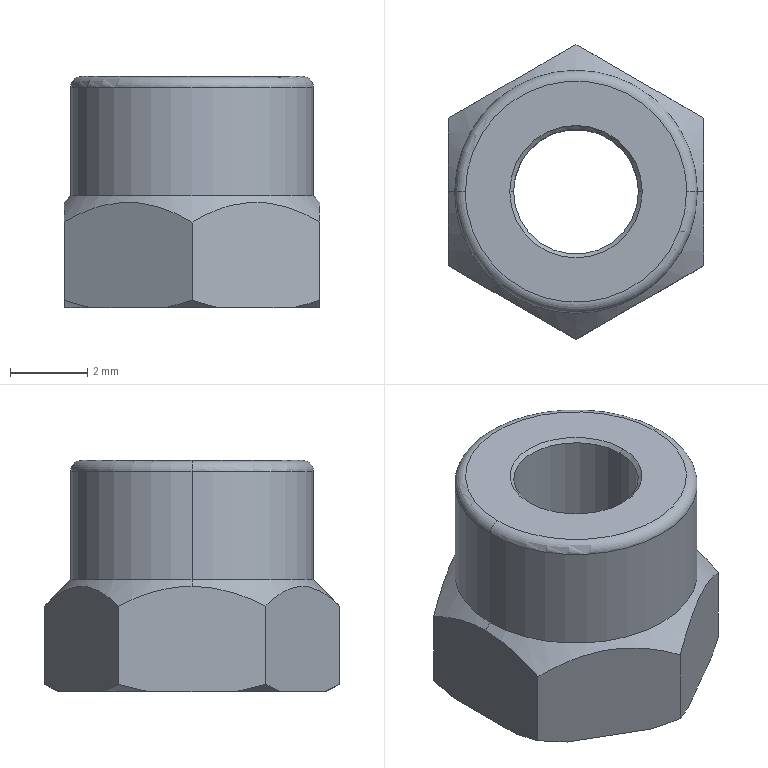Part | STEP file | 46A-01000LM15_Default<As Machined> | 1 solid | 26 faces | box 6.634 x 7.66 x 6 mm | volume 155.687 mm3 | cone 12 | plane 8 | cylinder 4 | torus 2 | commonest cylinder face diameters 3.242 x2 6.3 x2
STEP:
#1=CARTESIAN_POINT('',(1.621,0.,0.09881));
#2=VERTEX_POINT('',#1);
#3=CARTESIAN_POINT('',(-1.621,0.,0.09881));
#4=VERTEX_POINT('',#3);
#5=CARTESIAN_POINT('',(0.,0.,0.09881));
#6=DIRECTION('',(0.,0.,-1.));
#7=AXIS2_PLACEMENT_3D('',#5,#6,$);
#8=CIRCLE('',#7,1.621);
#9=EDGE_CURVE('',#2,#4,#8,.T.);
#10=ORIENTED_EDGE('',*,*,#9,.F.);
#11=CARTESIAN_POINT('',(1.72,0.,0.));
#12=VERTEX_POINT('',#11);
#13=CARTESIAN_POINT('',(353554.251,0.,-353552.531));
#14=DIRECTION('',(0.7071,0.,-0.7071));
#15=VECTOR('',#14,1.);
#16=LINE('',#13,#15);
#17=EDGE_CURVE('',#2,#12,#16,.T.);
#18=ORIENTED_EDGE('',*,*,#17,.T.);
#19=CARTESIAN_POINT('',(-1.72,0.,0.));
#20=VERTEX_POINT('',#19);
#21=CARTESIAN_POINT('',(0.,0.,0.));
#22=DIRECTION('',(0.,0.,-1.));
#23=AXIS2_PLACEMENT_3D('',#21,#22,$);
#24=CIRCLE('',#23,1.72);
#25=EDGE_CURVE('',#20,#12,#24,.F.);
#26=ORIENTED_EDGE('',*,*,#25,.F.);
#27=CARTESIAN_POINT('',(-353554.251,0.,-353552.531));
#28=DIRECTION('',(-0.7071,0.,-0.7071));
#29=VECTOR('',#28,1.);
#30=LINE('',#27,#29);
#31=EDGE_CURVE('',#4,#20,#30,.T.);
#32=ORIENTED_EDGE('',*,*,#31,.F.);
#33=EDGE_LOOP('',(#10,#18,#26,#32));
#34=FACE_OUTER_BOUND('',#33,.T.);
#35=CARTESIAN_POINT('',(0.,0.,0.));
#36=DIRECTION('',(0.,0.,-1.));
#37=DIRECTION('',(1.,0.,0.));
#38=AXIS2_PLACEMENT_3D('',#35,#36,#37);
#39=CONICAL_SURFACE('',#38,1.72,0.7854);
#40=ADVANCED_FACE('',(#34),#39,.F.);
#41=CARTESIAN_POINT('',(-1.621,0.,5.901));
#42=VERTEX_POINT('',#41);
#43=CARTESIAN_POINT('',(1.621,0.,5.901));
#44=VERTEX_POINT('',#43);
#45=CARTESIAN_POINT('',(0.,0.,5.901));
#46=DIRECTION('',(0.,0.,-1.));
#47=AXIS2_PLACEMENT_3D('',#45,#46,$);
#48=CIRCLE('',#47,1.621);
#49=EDGE_CURVE('',#42,#44,#48,.F.);
#50=ORIENTED_EDGE('',*,*,#49,.T.);
#51=CARTESIAN_POINT('',(1.621,0.,2.9));
#52=DIRECTION('',(0.,0.,-1.));
#53=VECTOR('',#52,1.);
#54=LINE('',#51,#53);
#55=EDGE_CURVE('',#44,#2,#54,.T.);
#56=ORIENTED_EDGE('',*,*,#55,.T.);
#57=ORIENTED_EDGE('',*,*,#9,.T.);
#58=CARTESIAN_POINT('',(-1.621,0.,2.9));
#59=DIRECTION('',(0.,0.,-1.));
#60=VECTOR('',#59,1.);
#61=LINE('',#58,#60);
#62=EDGE_CURVE('',#42,#4,#61,.T.);
#63=ORIENTED_EDGE('',*,*,#62,.F.);
#64=EDGE_LOOP('',(#50,#56,#57,#63));
#65=FACE_OUTER_BOUND('',#64,.T.);
#66=CARTESIAN_POINT('',(0.,0.,2.9));
#67=DIRECTION('',(0.,0.,-1.));
#68=DIRECTION('',(1.,0.,0.));
#69=AXIS2_PLACEMENT_3D('',#66,#67,#68);
#70=CYLINDRICAL_SURFACE('',#69,1.621);
#71=ADVANCED_FACE('',(#65),#70,.F.);
#72=ORIENTED_EDGE('',*,*,#17,.F.);
#73=CARTESIAN_POINT('',(0.,0.,0.09881));
#74=DIRECTION('',(0.,0.,-1.));
#75=AXIS2_PLACEMENT_3D('',#73,#74,$);
#76=CIRCLE('',#75,1.621);
#77=EDGE_CURVE('',#4,#2,#76,.T.);
#78=ORIENTED_EDGE('',*,*,#77,.F.);
#79=ORIENTED_EDGE('',*,*,#31,.T.);
#80=CARTESIAN_POINT('',(0.,0.,0.));
#81=DIRECTION('',(0.,0.,-1.));
#82=AXIS2_PLACEMENT_3D('',#80,#81,$);
#83=CIRCLE('',#82,1.72);
#84=EDGE_CURVE('',#12,#20,#83,.F.);
#85=ORIENTED_EDGE('',*,*,#84,.F.);
#86=EDGE_LOOP('',(#72,#78,#79,#85));
#87=FACE_OUTER_BOUND('',#86,.T.);
#88=CARTESIAN_POINT('',(0.,0.,0.));
#89=DIRECTION('',(0.,0.,-1.));
#90=DIRECTION('',(-1.,0.,0.));
#91=AXIS2_PLACEMENT_3D('',#88,#89,#90);
#92=CONICAL_SURFACE('',#91,1.72,0.7854);
#93=ADVANCED_FACE('',(#87),#92,.F.);
#94=CARTESIAN_POINT('',(-3.317,1.117,0.));
#95=VERTEX_POINT('',#94);
#96=CARTESIAN_POINT('',(-3.317,-1.117,0.));
#97=VERTEX_POINT('',#96);
#98=CARTESIAN_POINT('',(-3.317,0.,0.));
#99=DIRECTION('',(0.,-1.,0.));
#100=VECTOR('',#99,1.);
#101=LINE('',#98,#100);
#102=EDGE_CURVE('',#95,#97,#101,.T.);
#103=ORIENTED_EDGE('',*,*,#102,.F.);
#104=CARTESIAN_POINT('',(-2.626,2.314,0.));
#105=VERTEX_POINT('',#104);
#106=CARTESIAN_POINT('',(-0.000000015,0.00000001,0.));
#107=DIRECTION('',(0.,0.,-1.));
#108=AXIS2_PLACEMENT_3D('',#106,#107,$);
#109=CIRCLE('',#108,3.5);
#110=EDGE_CURVE('',#95,#105,#109,.T.);
#111=ORIENTED_EDGE('',*,*,#110,.T.);
#112=CARTESIAN_POINT('',(-0.6908,3.431,0.));
#113=VERTEX_POINT('',#112);
#114=CARTESIAN_POINT('',(-1.658,2.872,0.));
#115=DIRECTION('',(-0.866,-0.5,0.));
#116=VECTOR('',#115,1.);
#117=LINE('',#114,#116);
#118=EDGE_CURVE('',#113,#105,#117,.T.);
#119=ORIENTED_EDGE('',*,*,#118,.F.);
#120=CARTESIAN_POINT('',(0.6908,3.431,0.));
#121=VERTEX_POINT('',#120);
#122=CARTESIAN_POINT('',(-0.000000001,0.000000049,0.));
#123=DIRECTION('',(0.,0.,-1.));
#124=AXIS2_PLACEMENT_3D('',#122,#123,$);
#125=CIRCLE('',#124,3.5);
#126=EDGE_CURVE('',#113,#121,#125,.T.);
#127=ORIENTED_EDGE('',*,*,#126,.T.);
#128=CARTESIAN_POINT('',(2.626,2.314,0.));
#129=VERTEX_POINT('',#128);
#130=CARTESIAN_POINT('',(1.658,2.872,0.));
#131=DIRECTION('',(-0.866,0.5,0.));
#132=VECTOR('',#131,1.);
#133=LINE('',#130,#132);
#134=EDGE_CURVE('',#129,#121,#133,.T.);
#135=ORIENTED_EDGE('',*,*,#134,.F.);
#136=CARTESIAN_POINT('',(3.317,1.117,0.));
#137=VERTEX_POINT('',#136);
#138=CARTESIAN_POINT('',(0.000000016,0.00000001,0.));
#139=DIRECTION('',(0.,0.,-1.));
#140=AXIS2_PLACEMENT_3D('',#138,#139,$);
#141=CIRCLE('',#140,3.5);
#142=EDGE_CURVE('',#129,#137,#141,.T.);
#143=ORIENTED_EDGE('',*,*,#142,.T.);
#144=CARTESIAN_POINT('',(3.317,-1.117,0.));
#145=VERTEX_POINT('',#144);
#146=CARTESIAN_POINT('',(3.317,0.,0.));
#147=DIRECTION('',(0.,1.,0.));
#148=VECTOR('',#147,1.);
#149=LINE('',#146,#148);
#150=EDGE_CURVE('',#145,#137,#149,.T.);
#151=ORIENTED_EDGE('',*,*,#150,.F.);
#152=CARTESIAN_POINT('',(2.626,-2.314,0.));
#153=VERTEX_POINT('',#152);
#154=CARTESIAN_POINT('',(-0.000000025,0.000000014,0.));
#155=DIRECTION('',(0.,0.,-1.));
#156=AXIS2_PLACEMENT_3D('',#154,#155,$);
#157=CIRCLE('',#156,3.5);
#158=EDGE_CURVE('',#145,#153,#157,.T.);
#159=ORIENTED_EDGE('',*,*,#158,.T.);
#160=CARTESIAN_POINT('',(0.6908,-3.431,0.));
#161=VERTEX_POINT('',#160);
#162=CARTESIAN_POINT('',(1.658,-2.872,0.));
#163=DIRECTION('',(0.866,0.5,0.));
#164=VECTOR('',#163,1.);
#165=LINE('',#162,#164);
#166=EDGE_CURVE('',#161,#153,#165,.T.);
#167=ORIENTED_EDGE('',*,*,#166,.F.);
#168=CARTESIAN_POINT('',(-0.6908,-3.431,0.));
#169=VERTEX_POINT('',#168);
#170=CARTESIAN_POINT('',(-0.000000001,0.000000045,0.));
#171=DIRECTION('',(0.,0.,-1.));
#172=AXIS2_PLACEMENT_3D('',#170,#171,$);
#173=CIRCLE('',#172,3.5);
#174=EDGE_CURVE('',#161,#169,#173,.T.);
#175=ORIENTED_EDGE('',*,*,#174,.T.);
#176=CARTESIAN_POINT('',(-2.626,-2.314,0.));
#177=VERTEX_POINT('',#176);
#178=CARTESIAN_POINT('',(-1.658,-2.872,0.));
#179=DIRECTION('',(0.866,-0.5,0.));
#180=VECTOR('',#179,1.);
#181=LINE('',#178,#180);
#182=EDGE_CURVE('',#177,#169,#181,.T.);
#183=ORIENTED_EDGE('',*,*,#182,.F.);
#184=CARTESIAN_POINT('',(0.000000026,0.000000014,0.));
#185=DIRECTION('',(0.,0.,-1.));
#186=AXIS2_PLACEMENT_3D('',#184,#185,$);
#187=CIRCLE('',#186,3.5);
#188=EDGE_CURVE('',#177,#97,#187,.T.);
#189=ORIENTED_EDGE('',*,*,#188,.T.);
#190=EDGE_LOOP('',(#103,#111,#119,#127,#135,#143,#151,#159,#167,#175,#183,#189));
#191=FACE_OUTER_BOUND('',#190,.T.);
#192=ORIENTED_EDGE('',*,*,#25,.T.);
#193=ORIENTED_EDGE('',*,*,#84,.T.);
#194=EDGE_LOOP('',(#192,#193));
#195=FACE_BOUND('',#194,.T.);
#196=CARTESIAN_POINT('',(3.317,1.915,0.));
#197=DIRECTION('',(0.,0.,-1.));
#198=DIRECTION('',(-1.,0.,0.));
#199=AXIS2_PLACEMENT_3D('',#196,#197,#198);
#200=PLANE('',#199);
#201=ADVANCED_FACE('',(#191,#195),#200,.T.);
#202=ORIENTED_EDGE('',*,*,#49,.F.);
#203=CARTESIAN_POINT('',(-1.72,0.,6.));
#204=VERTEX_POINT('',#203);
#205=CARTESIAN_POINT('',(-353554.251,0.,353558.531));
#206=DIRECTION('',(-0.7071,0.,0.7071));
#207=VECTOR('',#206,1.);
#208=LINE('',#205,#207);
#209=EDGE_CURVE('',#42,#204,#208,.T.);
#210=ORIENTED_EDGE('',*,*,#209,.T.);
#211=CARTESIAN_POINT('',(1.72,0.,6.));
#212=VERTEX_POINT('',#211);
#213=CARTESIAN_POINT('',(0.,0.,6.));
#214=DIRECTION('',(0.,0.,1.));
#215=AXIS2_PLACEMENT_3D('',#213,#214,$);
#216=CIRCLE('',#215,1.72);
#217=EDGE_CURVE('',#212,#204,#216,.F.);
#218=ORIENTED_EDGE('',*,*,#217,.F.);
#219=CARTESIAN_POINT('',(353554.251,0.,353558.531));
#220=DIRECTION('',(0.7071,0.,0.7071));
#221=VECTOR('',#220,1.);
#222=LINE('',#219,#221);
#223=EDGE_CURVE('',#44,#212,#222,.T.);
#224=ORIENTED_EDGE('',*,*,#223,.F.);
#225=EDGE_LOOP('',(#202,#210,#218,#224));
#226=FACE_OUTER_BOUND('',#225,.T.);
#227=CARTESIAN_POINT('',(0.,0.,6.));
#228=DIRECTION('',(0.,0.,1.));
#229=DIRECTION('',(-1.,0.,0.));
#230=AXIS2_PLACEMENT_3D('',#227,#228,#229);
#231=CONICAL_SURFACE('',#230,1.72,0.7854);
#232=ADVANCED_FACE('',(#226),#231,.F.);
#233=ORIENTED_EDGE('',*,*,#55,.F.);
#234=CARTESIAN_POINT('',(0.,0.,5.901));
#235=DIRECTION('',(0.,0.,-1.));
#236=AXIS2_PLACEMENT_3D('',#234,#235,$);
#237=CIRCLE('',#236,1.621);
#238=EDGE_CURVE('',#44,#42,#237,.F.);
#239=ORIENTED_EDGE('',*,*,#238,.T.);
#240=ORIENTED_EDGE('',*,*,#62,.T.);
#241=ORIENTED_EDGE('',*,*,#77,.T.);
#242=EDGE_LOOP('',(#233,#239,#240,#241));
#243=FACE_OUTER_BOUND('',#242,.T.);
#244=CARTESIAN_POINT('',(0.,0.,2.9));
#245=DIRECTION('',(0.,0.,-1.));
#246=DIRECTION('',(-1.,0.,0.));
#247=AXIS2_PLACEMENT_3D('',#244,#245,#246);
#248=CYLINDRICAL_SURFACE('',#247,1.621);
#249=ADVANCED_FACE('',(#243),#248,.F.);
#250=CARTESIAN_POINT('',(-3.317,1.915,2.22));
#251=VERTEX_POINT('',#250);
#252=CARTESIAN_POINT('',(-3.317,0.,2.733));
#253=VERTEX_POINT('',#252);
#254=CARTESIAN_POINT('',(-3.317,1.915,2.22));
#255=CARTESIAN_POINT('',(-3.317,1.772,2.292));
#256=CARTESIAN_POINT('',(-3.317,1.627,2.359));
#257=CARTESIAN_POINT('',(-3.317,1.481,2.422));
#258=CARTESIAN_POINT('',(-3.317,1.18,2.537));
#259=CARTESIAN_POINT('',(-3.317,0.8711,2.626));
#260=CARTESIAN_POINT('',(-3.317,0.7149,2.662));
#261=CARTESIAN_POINT('',(-3.317,0.4792,2.704));
#262=CARTESIAN_POINT('',(-3.317,0.2406,2.726));
#263=CARTESIAN_POINT('',(-3.317,0.1605,2.731));
#264=CARTESIAN_POINT('',(-3.317,0.08038,2.733));
#265=CARTESIAN_POINT('',(-3.317,0.000000001,2.733));
#266=B_SPLINE_CURVE_WITH_KNOTS('',5,(#254,#255,#256,#257,#258,#259,#260,#261,#262,#263,#264,#265),.UNSPECIFIED.,.F.,.U.,(6,3,3,6),(0.,1.136,2.267,2.833),.UNSPECIFIED.);
#267=EDGE_CURVE('',#251,#253,#266,.T.);
#268=ORIENTED_EDGE('',*,*,#267,.F.);
#269=CARTESIAN_POINT('',(-3.317,1.915,0.1905));
#270=VERTEX_POINT('',#269);
#271=CARTESIAN_POINT('',(-3.317,1.915,1.205));
#272=DIRECTION('',(0.,0.,-1.));
#273=VECTOR('',#272,1.);
#274=LINE('',#271,#273);
#275=EDGE_CURVE('',#251,#270,#274,.T.);
#276=ORIENTED_EDGE('',*,*,#275,.T.);
#277=CARTESIAN_POINT('',(-3.317,1.117,0.));
#278=CARTESIAN_POINT('',(-3.317,1.279,0.02978));
#279=CARTESIAN_POINT('',(-3.317,1.439,0.06418));
#280=CARTESIAN_POINT('',(-3.317,1.599,0.1028));
#281=CARTESIAN_POINT('',(-3.317,1.757,0.145));
#282=CARTESIAN_POINT('',(-3.317,1.915,0.1905));
#283=B_SPLINE_CURVE_WITH_KNOTS('',5,(#277,#278,#279,#280,#281,#282),.UNSPECIFIED.,.F.,.U.,(6,6),(0.,1.16),.UNSPECIFIED.);
#284=EDGE_CURVE('',#95,#270,#283,.T.);
#285=ORIENTED_EDGE('',*,*,#284,.F.);
#286=ORIENTED_EDGE('',*,*,#102,.T.);
#287=CARTESIAN_POINT('',(-3.317,-1.915,0.1905));
#288=VERTEX_POINT('',#287);
#289=CARTESIAN_POINT('',(-3.317,-1.915,0.1905));
#290=CARTESIAN_POINT('',(-3.317,-1.757,0.145));
#291=CARTESIAN_POINT('',(-3.317,-1.598,0.1027));
#292=CARTESIAN_POINT('',(-3.317,-1.439,0.06406));
#293=CARTESIAN_POINT('',(-3.317,-1.278,0.02966));
#294=CARTESIAN_POINT('',(-3.317,-1.117,0.));
#295=B_SPLINE_CURVE_WITH_KNOTS('',5,(#289,#290,#291,#292,#293,#294),.UNSPECIFIED.,.F.,.U.,(6,6),(0.,1.16),.UNSPECIFIED.);
#296=EDGE_CURVE('',#288,#97,#295,.T.);
#297=ORIENTED_EDGE('',*,*,#296,.F.);
#298=CARTESIAN_POINT('',(-3.317,-1.915,2.22));
#299=VERTEX_POINT('',#298);
#300=CARTESIAN_POINT('',(-3.317,-1.915,1.205));
#301=DIRECTION('',(0.,0.,-1.));
#302=VECTOR('',#301,1.);
#303=LINE('',#300,#302);
#304=EDGE_CURVE('',#299,#288,#303,.T.);
#305=ORIENTED_EDGE('',*,*,#304,.F.);
#306=CARTESIAN_POINT('',(-3.317,0.000000001,2.733));
#307=CARTESIAN_POINT('',(-3.317,-0.08057,2.733));
#308=CARTESIAN_POINT('',(-3.317,-0.1611,2.731));
#309=CARTESIAN_POINT('',(-3.317,-0.2417,2.726));
#310=CARTESIAN_POINT('',(-3.317,-0.4814,2.704));
#311=CARTESIAN_POINT('',(-3.317,-0.7174,2.662));
#312=CARTESIAN_POINT('',(-3.317,-0.8725,2.625));
#313=CARTESIAN_POINT('',(-3.317,-1.179,2.537));
#314=CARTESIAN_POINT('',(-3.317,-1.479,2.422));
#315=CARTESIAN_POINT('',(-3.317,-1.627,2.359));
#316=CARTESIAN_POINT('',(-3.317,-1.772,2.291));
#317=CARTESIAN_POINT('',(-3.317,-1.915,2.22));
#318=B_SPLINE_CURVE_WITH_KNOTS('',5,(#306,#307,#308,#309,#310,#311,#312,#313,#314,#315,#316,#317),.UNSPECIFIED.,.F.,.U.,(6,3,3,6),(0.,0.5678,1.697,2.83),.UNSPECIFIED.);
#319=EDGE_CURVE('',#253,#299,#318,.T.);
#320=ORIENTED_EDGE('',*,*,#319,.F.);
#321=EDGE_LOOP('',(#268,#276,#285,#286,#297,#305,#320));
#322=FACE_OUTER_BOUND('',#321,.T.);
#323=CARTESIAN_POINT('',(-3.317,1.915,2.9));
#324=DIRECTION('',(1.,0.,0.));
#325=DIRECTION('',(0.,1.,0.));
#326=AXIS2_PLACEMENT_3D('',#323,#324,#325);
#327=PLANE('',#326);
#328=ADVANCED_FACE('',(#322),#327,.F.);
#329=CARTESIAN_POINT('',(-3.317,1.915,0.1905));
#330=CARTESIAN_POINT('',(-3.063,2.061,0.106));
#331=CARTESIAN_POINT('',(-2.838,2.192,0.04509));
#332=CARTESIAN_POINT('',(-2.626,2.314,0.));
#333=B_SPLINE_CURVE_WITH_KNOTS('',3,(#329,#330,#331,#332),.UNSPECIFIED.,.F.,.U.,(4,4),(0.,19.889),.UNSPECIFIED.);
#334=EDGE_CURVE('',#270,#105,#333,.T.);
#335=ORIENTED_EDGE('',*,*,#334,.T.);
#336=ORIENTED_EDGE('',*,*,#110,.F.);
#337=ORIENTED_EDGE('',*,*,#284,.T.);
#338=EDGE_LOOP('',(#335,#336,#337));
#339=FACE_OUTER_BOUND('',#338,.T.);
#340=CARTESIAN_POINT('',(0.,0.,0.));
#341=DIRECTION('',(0.,0.,1.));
#342=DIRECTION('',(1.,0.,0.));
#343=AXIS2_PLACEMENT_3D('',#340,#341,#342);
#344=CONICAL_SURFACE('',#343,3.5,1.047);
#345=ADVANCED_FACE('',(#339),#344,.T.);
#346=CARTESIAN_POINT('',(0.,3.83,2.22));
#347=VERTEX_POINT('',#346);
#348=CARTESIAN_POINT('',(0.,3.83,2.22));
#349=CARTESIAN_POINT('',(-0.1625,3.736,2.314));
#350=CARTESIAN_POINT('',(-0.3274,3.641,2.401));
#351=CARTESIAN_POINT('',(-0.4944,3.545,2.478));
#352=CARTESIAN_POINT('',(-0.7397,3.403,2.575));
#353=CARTESIAN_POINT('',(-0.9915,3.258,2.647));
#354=CARTESIAN_POINT('',(-1.069,3.213,2.666));
#355=CARTESIAN_POINT('',(-1.221,3.125,2.698));
#356=CARTESIAN_POINT('',(-1.376,3.036,2.719));
#357=CARTESIAN_POINT('',(-1.452,2.992,2.726));
#358=CARTESIAN_POINT('',(-1.684,2.858,2.74));
#359=CARTESIAN_POINT('',(-1.916,2.724,2.727));
#360=CARTESIAN_POINT('',(-2.072,2.633,2.705));
#361=CARTESIAN_POINT('',(-2.422,2.431,2.632));
#362=CARTESIAN_POINT('',(-2.763,2.235,2.506));
#363=CARTESIAN_POINT('',(-2.953,2.125,2.42));
#364=CARTESIAN_POINT('',(-3.137,2.019,2.324));
#365=CARTESIAN_POINT('',(-3.317,1.915,2.22));
#366=B_SPLINE_CURVE_WITH_KNOTS('',5,(#348,#349,#350,#351,#352,#353,#354,#355,#356,#357,#358,#359,#360,#361,#362,#363,#364,#365),.UNSPECIFIED.,.F.,.U.,(6,3,3,3,3,6),(0.,1.482,2.129,2.752,4.018,5.657),.UNSPECIFIED.);
#367=EDGE_CURVE('',#347,#251,#366,.T.);
#368=ORIENTED_EDGE('',*,*,#367,.F.);
#369=CARTESIAN_POINT('',(0.,3.83,0.1905));
#370=VERTEX_POINT('',#369);
#371=CARTESIAN_POINT('',(0.,3.83,1.205));
#372=DIRECTION('',(0.,0.,-1.));
#373=VECTOR('',#372,1.);
#374=LINE('',#371,#373);
#375=EDGE_CURVE('',#347,#370,#374,.T.);
#376=ORIENTED_EDGE('',*,*,#375,.T.);
#377=CARTESIAN_POINT('',(-0.6908,3.431,0.));
#378=CARTESIAN_POINT('',(-0.5511,3.512,0.02974));
#379=CARTESIAN_POINT('',(-0.4122,3.592,0.06411));
#380=CARTESIAN_POINT('',(-0.274,3.672,0.1027));
#381=CARTESIAN_POINT('',(-0.1366,3.751,0.145));
#382=CARTESIAN_POINT('',(0.,3.83,0.1905));
#383=B_SPLINE_CURVE_WITH_KNOTS('',5,(#377,#378,#379,#380,#381,#382),.UNSPECIFIED.,.F.,.U.,(6,6),(0.,1.16),.UNSPECIFIED.);
#384=EDGE_CURVE('',#113,#370,#383,.T.);
#385=ORIENTED_EDGE('',*,*,#384,.F.);
#386=ORIENTED_EDGE('',*,*,#118,.T.);
#387=ORIENTED_EDGE('',*,*,#334,.F.);
#388=ORIENTED_EDGE('',*,*,#275,.F.);
#389=EDGE_LOOP('',(#368,#376,#385,#386,#387,#388));
#390=FACE_OUTER_BOUND('',#389,.T.);
#391=CARTESIAN_POINT('',(0.,3.83,2.9));
#392=DIRECTION('',(0.5,-0.866,0.));
#393=DIRECTION('',(0.866,0.5,0.));
#394=AXIS2_PLACEMENT_3D('',#391,#392,#393);
#395=PLANE('',#394);
#396=ADVANCED_FACE('',(#390),#395,.F.);
#397=CARTESIAN_POINT('',(0.,3.83,0.1905));
#398=CARTESIAN_POINT('',(0.2536,3.684,0.106));
#399=CARTESIAN_POINT('',(0.479,3.553,0.04509));
#400=CARTESIAN_POINT('',(0.6908,3.431,0.));
#401=B_SPLINE_CURVE_WITH_KNOTS('',3,(#397,#398,#399,#400),.UNSPECIFIED.,.F.,.U.,(4,4),(0.,19.889),.UNSPECIFIED.);
#402=EDGE_CURVE('',#370,#121,#401,.T.);
#403=ORIENTED_EDGE('',*,*,#402,.T.);
#404=ORIENTED_EDGE('',*,*,#126,.F.);
#405=ORIENTED_EDGE('',*,*,#384,.T.);
#406=EDGE_LOOP('',(#403,#404,#405));
#407=FACE_OUTER_BOUND('',#406,.T.);
#408=CARTESIAN_POINT('',(0.,0.,0.));
#409=DIRECTION('',(0.,0.,1.));
#410=DIRECTION('',(1.,0.,0.));
#411=AXIS2_PLACEMENT_3D('',#408,#409,#410);
#412=CONICAL_SURFACE('',#411,3.5,1.047);
#413=ADVANCED_FACE('',(#407),#412,.T.);
#414=CARTESIAN_POINT('',(3.317,1.915,2.22));
#415=VERTEX_POINT('',#414);
#416=CARTESIAN_POINT('',(3.317,1.915,2.22));
#417=CARTESIAN_POINT('',(3.154,2.009,2.314));
#418=CARTESIAN_POINT('',(2.989,2.104,2.401));
#419=CARTESIAN_POINT('',(2.822,2.2,2.478));
#420=CARTESIAN_POINT('',(2.577,2.342,2.575));
#421=CARTESIAN_POINT('',(2.325,2.487,2.647));
#422=CARTESIAN_POINT('',(2.248,2.532,2.666));
#423=CARTESIAN_POINT('',(2.096,2.62,2.698));
#424=CARTESIAN_POINT('',(1.941,2.709,2.719));
#425=CARTESIAN_POINT('',(1.865,2.753,2.726));
#426=CARTESIAN_POINT('',(1.633,2.887,2.74));
#427=CARTESIAN_POINT('',(1.401,3.021,2.727));
#428=CARTESIAN_POINT('',(1.244,3.112,2.705));
#429=CARTESIAN_POINT('',(0.8945,3.314,2.632));
#430=CARTESIAN_POINT('',(0.5541,3.51,2.506));
#431=CARTESIAN_POINT('',(0.3638,3.62,2.42));
#432=CARTESIAN_POINT('',(0.1798,3.726,2.324));
#433=CARTESIAN_POINT('',(0.,3.83,2.22));
#434=B_SPLINE_CURVE_WITH_KNOTS('',5,(#416,#417,#418,#419,#420,#421,#422,#423,#424,#425,#426,#427,#428,#429,#430,#431,#432,#433),.UNSPECIFIED.,.F.,.U.,(6,3,3,3,3,6),(0.,1.482,2.129,2.752,4.018,5.657),.UNSPECIFIED.);
#435=EDGE_CURVE('',#415,#347,#434,.T.);
#436=ORIENTED_EDGE('',*,*,#435,.F.);
#437=CARTESIAN_POINT('',(3.317,1.915,0.1905));
#438=VERTEX_POINT('',#437);
#439=CARTESIAN_POINT('',(3.317,1.915,1.205));
#440=DIRECTION('',(0.,0.,-1.));
#441=VECTOR('',#440,1.);
#442=LINE('',#439,#441);
#443=EDGE_CURVE('',#415,#438,#442,.T.);
#444=ORIENTED_EDGE('',*,*,#443,.T.);
#445=CARTESIAN_POINT('',(2.626,2.314,0.));
#446=CARTESIAN_POINT('',(2.766,2.233,0.02974));
#447=CARTESIAN_POINT('',(2.905,2.153,0.06411));
#448=CARTESIAN_POINT('',(3.043,2.073,0.1027));
#449=CARTESIAN_POINT('',(3.18,1.994,0.145));
#450=CARTESIAN_POINT('',(3.317,1.915,0.1905));
#451=B_SPLINE_CURVE_WITH_KNOTS('',5,(#445,#446,#447,#448,#449,#450),.UNSPECIFIED.,.F.,.U.,(6,6),(0.,1.16),.UNSPECIFIED.);
#452=EDGE_CURVE('',#129,#438,#451,.T.);
#453=ORIENTED_EDGE('',*,*,#452,.F.);
#454=ORIENTED_EDGE('',*,*,#134,.T.);
#455=ORIENTED_EDGE('',*,*,#402,.F.);
#456=ORIENTED_EDGE('',*,*,#375,.F.);
#457=EDGE_LOOP('',(#436,#444,#453,#454,#455,#456));
#458=FACE_OUTER_BOUND('',#457,.T.);
#459=CARTESIAN_POINT('',(3.317,1.915,2.9));
#460=DIRECTION('',(-0.5,-0.866,0.));
#461=DIRECTION('',(0.866,-0.5,0.));
#462=AXIS2_PLACEMENT_3D('',#459,#460,#461);
#463=PLANE('',#462);
#464=ADVANCED_FACE('',(#458),#463,.F.);
#465=ORIENTED_EDGE('',*,*,#452,.T.);
#466=CARTESIAN_POINT('',(3.317,1.915,0.1905));
#467=CARTESIAN_POINT('',(3.317,1.622,0.106));
#468=CARTESIAN_POINT('',(3.317,1.362,0.04509));
#469=CARTESIAN_POINT('',(3.317,1.117,0.));
#470=B_SPLINE_CURVE_WITH_KNOTS('',3,(#466,#467,#468,#469),.UNSPECIFIED.,.F.,.U.,(4,4),(0.,19.889),.UNSPECIFIED.);
#471=EDGE_CURVE('',#438,#137,#470,.T.);
#472=ORIENTED_EDGE('',*,*,#471,.T.);
#473=ORIENTED_EDGE('',*,*,#142,.F.);
#474=EDGE_LOOP('',(#465,#472,#473));
#475=FACE_OUTER_BOUND('',#474,.T.);
#476=CARTESIAN_POINT('',(0.,0.,0.));
#477=DIRECTION('',(0.,0.,1.));
#478=DIRECTION('',(1.,0.,0.));
#479=AXIS2_PLACEMENT_3D('',#476,#477,#478);
#480=CONICAL_SURFACE('',#479,3.5,1.047);
#481=ADVANCED_FACE('',(#475),#480,.T.);
#482=CARTESIAN_POINT('',(3.317,-1.915,2.22));
#483=VERTEX_POINT('',#482);
#484=CARTESIAN_POINT('',(3.317,0.,2.733));
#485=VERTEX_POINT('',#484);
#486=CARTESIAN_POINT('',(3.317,-1.915,2.22));
#487=CARTESIAN_POINT('',(3.317,-1.772,2.291));
#488=CARTESIAN_POINT('',(3.317,-1.627,2.359));
#489=CARTESIAN_POINT('',(3.317,-1.479,2.422));
#490=CARTESIAN_POINT('',(3.317,-1.179,2.537));
#491=CARTESIAN_POINT('',(3.317,-0.8725,2.625));
#492=CARTESIAN_POINT('',(3.317,-0.7174,2.662));
#493=CARTESIAN_POINT('',(3.317,-0.4814,2.704));
#494=CARTESIAN_POINT('',(3.317,-0.2417,2.726));
#495=CARTESIAN_POINT('',(3.317,-0.1611,2.731));
#496=CARTESIAN_POINT('',(3.317,-0.08057,2.733));
#497=CARTESIAN_POINT('',(3.317,-0.000000001,2.733));
#498=B_SPLINE_CURVE_WITH_KNOTS('',5,(#486,#487,#488,#489,#490,#491,#492,#493,#494,#495,#496,#497),.UNSPECIFIED.,.F.,.U.,(6,3,3,6),(0.,1.133,2.262,2.83),.UNSPECIFIED.);
#499=EDGE_CURVE('',#483,#485,#498,.T.);
#500=ORIENTED_EDGE('',*,*,#499,.F.);
#501=CARTESIAN_POINT('',(3.317,-1.915,0.1905));
#502=VERTEX_POINT('',#501);
#503=CARTESIAN_POINT('',(3.317,-1.915,1.205));
#504=DIRECTION('',(0.,0.,-1.));
#505=VECTOR('',#504,1.);
#506=LINE('',#503,#505);
#507=EDGE_CURVE('',#483,#502,#506,.T.);
#508=ORIENTED_EDGE('',*,*,#507,.T.);
#509=CARTESIAN_POINT('',(3.317,-1.117,0.));
#510=CARTESIAN_POINT('',(3.317,-1.279,0.02978));
#511=CARTESIAN_POINT('',(3.317,-1.439,0.06418));
#512=CARTESIAN_POINT('',(3.317,-1.599,0.1028));
#513=CARTESIAN_POINT('',(3.317,-1.757,0.145));
#514=CARTESIAN_POINT('',(3.317,-1.915,0.1905));
#515=B_SPLINE_CURVE_WITH_KNOTS('',5,(#509,#510,#511,#512,#513,#514),.UNSPECIFIED.,.F.,.U.,(6,6),(0.,1.16),.UNSPECIFIED.);
#516=EDGE_CURVE('',#145,#502,#515,.T.);
#517=ORIENTED_EDGE('',*,*,#516,.F.);
#518=ORIENTED_EDGE('',*,*,#150,.T.);
#519=ORIENTED_EDGE('',*,*,#471,.F.);
#520=ORIENTED_EDGE('',*,*,#443,.F.);
#521=CARTESIAN_POINT('',(3.317,-0.000000001,2.733));
#522=CARTESIAN_POINT('',(3.317,0.1604,2.733));
#523=CARTESIAN_POINT('',(3.317,0.32,2.723));
#524=CARTESIAN_POINT('',(3.317,0.4792,2.704));
#525=CARTESIAN_POINT('',(3.317,0.7936,2.648));
#526=CARTESIAN_POINT('',(3.317,1.102,2.56));
#527=CARTESIAN_POINT('',(3.317,1.256,2.508));
#528=CARTESIAN_POINT('',(3.317,1.48,2.421));
#529=CARTESIAN_POINT('',(3.317,1.7,2.324));
#530=CARTESIAN_POINT('',(3.317,1.772,2.29));
#531=CARTESIAN_POINT('',(3.317,1.844,2.256));
#532=CARTESIAN_POINT('',(3.317,1.915,2.22));
#533=B_SPLINE_CURVE_WITH_KNOTS('',5,(#521,#522,#523,#524,#525,#526,#527,#528,#529,#530,#531,#532),.UNSPECIFIED.,.F.,.U.,(6,3,3,6),(0.,1.131,2.264,2.83),.UNSPECIFIED.);
#534=EDGE_CURVE('',#485,#415,#533,.T.);
#535=ORIENTED_EDGE('',*,*,#534,.F.);
#536=EDGE_LOOP('',(#500,#508,#517,#518,#519,#520,#535));
#537=FACE_OUTER_BOUND('',#536,.T.);
#538=CARTESIAN_POINT('',(3.317,-1.915,2.9));
#539=DIRECTION('',(-1.,0.,0.));
#540=DIRECTION('',(0.,-1.,0.));
#541=AXIS2_PLACEMENT_3D('',#538,#539,#540);
#542=PLANE('',#541);
#543=ADVANCED_FACE('',(#537),#542,.F.);
#544=CARTESIAN_POINT('',(3.317,-1.915,0.1905));
#545=CARTESIAN_POINT('',(3.063,-2.061,0.106));
#546=CARTESIAN_POINT('',(2.838,-2.192,0.04509));
#547=CARTESIAN_POINT('',(2.626,-2.314,0.));
#548=B_SPLINE_CURVE_WITH_KNOTS('',3,(#544,#545,#546,#547),.UNSPECIFIED.,.F.,.U.,(4,4),(0.,19.889),.UNSPECIFIED.);
#549=EDGE_CURVE('',#502,#153,#548,.T.);
#550=ORIENTED_EDGE('',*,*,#549,.T.);
#551=ORIENTED_EDGE('',*,*,#158,.F.);
#552=ORIENTED_EDGE('',*,*,#516,.T.);
#553=EDGE_LOOP('',(#550,#551,#552));
#554=FACE_OUTER_BOUND('',#553,.T.);
#555=CARTESIAN_POINT('',(0.,0.,0.));
#556=DIRECTION('',(0.,0.,1.));
#557=DIRECTION('',(-1.,0.,0.));
#558=AXIS2_PLACEMENT_3D('',#555,#556,#557);
#559=CONICAL_SURFACE('',#558,3.5,1.047);
#560=ADVANCED_FACE('',(#554),#559,.T.);
#561=CARTESIAN_POINT('',(0.,-3.83,2.22));
#562=VERTEX_POINT('',#561);
#563=CARTESIAN_POINT('',(0.,-3.83,2.22));
#564=CARTESIAN_POINT('',(0.1625,-3.736,2.314));
#565=CARTESIAN_POINT('',(0.3274,-3.641,2.401));
#566=CARTESIAN_POINT('',(0.4944,-3.545,2.478));
#567=CARTESIAN_POINT('',(0.7397,-3.403,2.575));
#568=CARTESIAN_POINT('',(0.9915,-3.258,2.647));
#569=CARTESIAN_POINT('',(1.069,-3.213,2.666));
#570=CARTESIAN_POINT('',(1.221,-3.125,2.698));
#571=CARTESIAN_POINT('',(1.376,-3.036,2.719));
#572=CARTESIAN_POINT('',(1.452,-2.992,2.726));
#573=CARTESIAN_POINT('',(1.684,-2.858,2.74));
#574=CARTESIAN_POINT('',(1.916,-2.724,2.727));
#575=CARTESIAN_POINT('',(2.072,-2.633,2.705));
#576=CARTESIAN_POINT('',(2.422,-2.431,2.632));
#577=CARTESIAN_POINT('',(2.763,-2.235,2.506));
#578=CARTESIAN_POINT('',(2.953,-2.125,2.42));
#579=CARTESIAN_POINT('',(3.137,-2.019,2.324));
#580=CARTESIAN_POINT('',(3.317,-1.915,2.22));
#581=B_SPLINE_CURVE_WITH_KNOTS('',5,(#563,#564,#565,#566,#567,#568,#569,#570,#571,#572,#573,#574,#575,#576,#577,#578,#579,#580),.UNSPECIFIED.,.F.,.U.,(6,3,3,3,3,6),(0.,1.482,2.129,2.752,4.018,5.657),.UNSPECIFIED.);
#582=EDGE_CURVE('',#562,#483,#581,.T.);
#583=ORIENTED_EDGE('',*,*,#582,.F.);
#584=CARTESIAN_POINT('',(0.,-3.83,0.1905));
#585=VERTEX_POINT('',#584);
#586=CARTESIAN_POINT('',(0.,-3.83,1.205));
#587=DIRECTION('',(0.,0.,-1.));
#588=VECTOR('',#587,1.);
#589=LINE('',#586,#588);
#590=EDGE_CURVE('',#562,#585,#589,.T.);
#591=ORIENTED_EDGE('',*,*,#590,.T.);
#592=CARTESIAN_POINT('',(0.6908,-3.431,0.));
#593=CARTESIAN_POINT('',(0.5511,-3.512,0.02974));
#594=CARTESIAN_POINT('',(0.4122,-3.592,0.06411));
#595=CARTESIAN_POINT('',(0.274,-3.672,0.1027));
#596=CARTESIAN_POINT('',(0.1366,-3.751,0.145));
#597=CARTESIAN_POINT('',(0.,-3.83,0.1905));
#598=B_SPLINE_CURVE_WITH_KNOTS('',5,(#592,#593,#594,#595,#596,#597),.UNSPECIFIED.,.F.,.U.,(6,6),(0.,1.16),.UNSPECIFIED.);
#599=EDGE_CURVE('',#161,#585,#598,.T.);
#600=ORIENTED_EDGE('',*,*,#599,.F.);
#601=ORIENTED_EDGE('',*,*,#166,.T.);
#602=ORIENTED_EDGE('',*,*,#549,.F.);
#603=ORIENTED_EDGE('',*,*,#507,.F.);
#604=EDGE_LOOP('',(#583,#591,#600,#601,#602,#603));
#605=FACE_OUTER_BOUND('',#604,.T.);
#606=CARTESIAN_POINT('',(0.,-3.83,2.9));
#607=DIRECTION('',(-0.5,0.866,0.));
#608=DIRECTION('',(-0.866,-0.5,0.));
#609=AXIS2_PLACEMENT_3D('',#606,#607,#608);
#610=PLANE('',#609);
#611=ADVANCED_FACE('',(#605),#610,.F.);
#612=CARTESIAN_POINT('',(0.,-3.83,0.1905));
#613=CARTESIAN_POINT('',(-0.2536,-3.684,0.106));
#614=CARTESIAN_POINT('',(-0.479,-3.553,0.04509));
#615=CARTESIAN_POINT('',(-0.6908,-3.431,0.));
#616=B_SPLINE_CURVE_WITH_KNOTS('',3,(#612,#613,#614,#615),.UNSPECIFIED.,.F.,.U.,(4,4),(0.,19.889),.UNSPECIFIED.);
#617=EDGE_CURVE('',#585,#169,#616,.T.);
#618=ORIENTED_EDGE('',*,*,#617,.T.);
#619=ORIENTED_EDGE('',*,*,#174,.F.);
#620=ORIENTED_EDGE('',*,*,#599,.T.);
#621=EDGE_LOOP('',(#618,#619,#620));
#622=FACE_OUTER_BOUND('',#621,.T.);
#623=CARTESIAN_POINT('',(0.,0.,0.));
#624=DIRECTION('',(0.,0.,1.));
#625=DIRECTION('',(-1.,0.,0.));
#626=AXIS2_PLACEMENT_3D('',#623,#624,#625);
#627=CONICAL_SURFACE('',#626,3.5,1.047);
#628=ADVANCED_FACE('',(#622),#627,.T.);
#629=CARTESIAN_POINT('',(-3.317,-1.915,2.22));
#630=CARTESIAN_POINT('',(-3.154,-2.009,2.314));
#631=CARTESIAN_POINT('',(-2.989,-2.104,2.401));
#632=CARTESIAN_POINT('',(-2.822,-2.2,2.478));
#633=CARTESIAN_POINT('',(-2.577,-2.342,2.575));
#634=CARTESIAN_POINT('',(-2.325,-2.487,2.647));
#635=CARTESIAN_POINT('',(-2.248,-2.532,2.666));
#636=CARTESIAN_POINT('',(-2.096,-2.62,2.698));
#637=CARTESIAN_POINT('',(-1.941,-2.709,2.719));
#638=CARTESIAN_POINT('',(-1.865,-2.753,2.726));
#639=CARTESIAN_POINT('',(-1.633,-2.887,2.74));
#640=CARTESIAN_POINT('',(-1.401,-3.021,2.727));
#641=CARTESIAN_POINT('',(-1.244,-3.112,2.705));
#642=CARTESIAN_POINT('',(-0.8945,-3.314,2.632));
#643=CARTESIAN_POINT('',(-0.5541,-3.51,2.506));
#644=CARTESIAN_POINT('',(-0.3638,-3.62,2.42));
#645=CARTESIAN_POINT('',(-0.1798,-3.726,2.324));
#646=CARTESIAN_POINT('',(0.,-3.83,2.22));
#647=B_SPLINE_CURVE_WITH_KNOTS('',5,(#629,#630,#631,#632,#633,#634,#635,#636,#637,#638,#639,#640,#641,#642,#643,#644,#645,#646),.UNSPECIFIED.,.F.,.U.,(6,3,3,3,3,6),(0.,1.482,2.129,2.752,4.018,5.657),.UNSPECIFIED.);
#648=EDGE_CURVE('',#299,#562,#647,.T.);
#649=ORIENTED_EDGE('',*,*,#648,.F.);
#650=ORIENTED_EDGE('',*,*,#304,.T.);
#651=CARTESIAN_POINT('',(-2.626,-2.314,0.));
#652=CARTESIAN_POINT('',(-2.766,-2.233,0.02974));
#653=CARTESIAN_POINT('',(-2.905,-2.153,0.06411));
#654=CARTESIAN_POINT('',(-3.043,-2.073,0.1027));
#655=CARTESIAN_POINT('',(-3.18,-1.994,0.145));
#656=CARTESIAN_POINT('',(-3.317,-1.915,0.1905));
#657=B_SPLINE_CURVE_WITH_KNOTS('',5,(#651,#652,#653,#654,#655,#656),.UNSPECIFIED.,.F.,.U.,(6,6),(0.,1.16),.UNSPECIFIED.);
#658=EDGE_CURVE('',#177,#288,#657,.T.);
#659=ORIENTED_EDGE('',*,*,#658,.F.);
#660=ORIENTED_EDGE('',*,*,#182,.T.);
#661=ORIENTED_EDGE('',*,*,#617,.F.);
#662=ORIENTED_EDGE('',*,*,#590,.F.);
#663=EDGE_LOOP('',(#649,#650,#659,#660,#661,#662));
#664=FACE_OUTER_BOUND('',#663,.T.);
#665=CARTESIAN_POINT('',(-3.317,-1.915,2.9));
#666=DIRECTION('',(0.5,0.866,0.));
#667=DIRECTION('',(-0.866,0.5,0.));
#668=AXIS2_PLACEMENT_3D('',#665,#666,#667);
#669=PLANE('',#668);
#670=ADVANCED_FACE('',(#664),#669,.F.);
#671=ORIENTED_EDGE('',*,*,#296,.T.);
#672=ORIENTED_EDGE('',*,*,#188,.F.);
#673=ORIENTED_EDGE('',*,*,#658,.T.);
#674=EDGE_LOOP('',(#671,#672,#673));
#675=FACE_OUTER_BOUND('',#674,.T.);
#676=CARTESIAN_POINT('',(0.,0.,0.));
#677=DIRECTION('',(0.,0.,1.));
#678=DIRECTION('',(-1.,0.,0.));
#679=AXIS2_PLACEMENT_3D('',#676,#677,#678);
#680=CONICAL_SURFACE('',#679,3.5,1.047);
#681=ADVANCED_FACE('',(#675),#680,.T.);
#682=ORIENTED_EDGE('',*,*,#209,.F.);
#683=ORIENTED_EDGE('',*,*,#238,.F.);
#684=ORIENTED_EDGE('',*,*,#223,.T.);
#685=CARTESIAN_POINT('',(0.,0.,6.));
#686=DIRECTION('',(0.,0.,1.));
#687=AXIS2_PLACEMENT_3D('',#685,#686,$);
#688=CIRCLE('',#687,1.72);
#689=EDGE_CURVE('',#204,#212,#688,.F.);
#690=ORIENTED_EDGE('',*,*,#689,.F.);
#691=EDGE_LOOP('',(#682,#683,#684,#690));
#692=FACE_OUTER_BOUND('',#691,.T.);
#693=CARTESIAN_POINT('',(0.,0.,6.));
#694=DIRECTION('',(0.,0.,1.));
#695=DIRECTION('',(1.,0.,0.));
#696=AXIS2_PLACEMENT_3D('',#693,#694,#695);
#697=CONICAL_SURFACE('',#696,1.72,0.7854);
#698=ADVANCED_FACE('',(#692),#697,.F.);
#699=CARTESIAN_POINT('',(-2.87,0.,6.));
#700=VERTEX_POINT('',#699);
#701=CARTESIAN_POINT('',(2.87,0.,6.));
#702=VERTEX_POINT('',#701);
#703=CARTESIAN_POINT('',(-2.87,0.000000001,6.));
#704=CARTESIAN_POINT('',(-2.87,0.332,6.));
#705=CARTESIAN_POINT('',(-2.822,0.6639,6.));
#706=CARTESIAN_POINT('',(-2.726,0.9867,6.));
#707=CARTESIAN_POINT('',(-2.443,1.595,6.));
#708=CARTESIAN_POINT('',(-2.,2.099,6.));
#709=CARTESIAN_POINT('',(-1.743,2.316,6.));
#710=CARTESIAN_POINT('',(-1.174,2.671,6.));
#711=CARTESIAN_POINT('',(-0.5276,2.851,6.));
#712=CARTESIAN_POINT('',(-0.1935,2.893,6.));
#713=CARTESIAN_POINT('',(0.4772,2.879,6.));
#714=CARTESIAN_POINT('',(1.116,2.675,6.));
#715=CARTESIAN_POINT('',(1.419,2.528,6.));
#716=CARTESIAN_POINT('',(1.973,2.15,6.));
#717=CARTESIAN_POINT('',(2.397,1.63,6.));
#718=CARTESIAN_POINT('',(2.57,1.341,6.));
#719=CARTESIAN_POINT('',(2.754,0.8976,6.));
#720=CARTESIAN_POINT('',(2.843,0.4298,6.));
#721=CARTESIAN_POINT('',(2.861,0.2864,6.));
#722=CARTESIAN_POINT('',(2.87,0.1432,6.));
#723=CARTESIAN_POINT('',(2.87,0.000000001,6.));
#724=B_SPLINE_CURVE_WITH_KNOTS('',5,(#703,#704,#705,#706,#707,#708,#709,#710,#711,#712,#713,#714,#715,#716,#717,#718,#719,#720,#721,#722,#723),.UNSPECIFIED.,.F.,.U.,(6,3,3,3,3,3,6),(0.,2.347,4.695,7.042,9.39,11.737,12.75),.UNSPECIFIED.);
#725=EDGE_CURVE('',#700,#702,#724,.T.);
#726=ORIENTED_EDGE('',*,*,#725,.F.);
#727=CARTESIAN_POINT('',(2.87,0.000000001,6.));
#728=CARTESIAN_POINT('',(2.87,-0.332,6.));
#729=CARTESIAN_POINT('',(2.822,-0.6639,6.));
#730=CARTESIAN_POINT('',(2.726,-0.9867,6.));
#731=CARTESIAN_POINT('',(2.443,-1.595,6.));
#732=CARTESIAN_POINT('',(2.,-2.099,6.));
#733=CARTESIAN_POINT('',(1.743,-2.316,6.));
#734=CARTESIAN_POINT('',(1.174,-2.671,6.));
#735=CARTESIAN_POINT('',(0.5276,-2.851,6.));
#736=CARTESIAN_POINT('',(0.1935,-2.893,6.));
#737=CARTESIAN_POINT('',(-0.4772,-2.879,6.));
#738=CARTESIAN_POINT('',(-1.116,-2.675,6.));
#739=CARTESIAN_POINT('',(-1.419,-2.528,6.));
#740=CARTESIAN_POINT('',(-1.973,-2.15,6.));
#741=CARTESIAN_POINT('',(-2.397,-1.63,6.));
#742=CARTESIAN_POINT('',(-2.57,-1.341,6.));
#743=CARTESIAN_POINT('',(-2.754,-0.8976,6.));
#744=CARTESIAN_POINT('',(-2.843,-0.4298,6.));
#745=CARTESIAN_POINT('',(-2.861,-0.2864,6.));
#746=CARTESIAN_POINT('',(-2.87,-0.1432,6.));
#747=CARTESIAN_POINT('',(-2.87,0.000000001,6.));
#748=B_SPLINE_CURVE_WITH_KNOTS('',5,(#727,#728,#729,#730,#731,#732,#733,#734,#735,#736,#737,#738,#739,#740,#741,#742,#743,#744,#745,#746,#747),.UNSPECIFIED.,.F.,.U.,(6,3,3,3,3,3,6),(0.,2.347,4.695,7.042,9.39,11.737,12.75),.UNSPECIFIED.);
#749=EDGE_CURVE('',#702,#700,#748,.T.);
#750=ORIENTED_EDGE('',*,*,#749,.F.);
#751=EDGE_LOOP('',(#726,#750));
#752=FACE_OUTER_BOUND('',#751,.T.);
#753=ORIENTED_EDGE('',*,*,#217,.T.);
#754=ORIENTED_EDGE('',*,*,#689,.T.);
#755=EDGE_LOOP('',(#753,#754));
#756=FACE_BOUND('',#755,.T.);
#757=CARTESIAN_POINT('',(0.,2.87,6.));
#758=DIRECTION('',(0.,0.,1.));
#759=DIRECTION('',(1.,0.,0.));
#760=AXIS2_PLACEMENT_3D('',#757,#758,#759);
#761=PLANE('',#760);
#762=ADVANCED_FACE('',(#752,#756),#761,.T.);
#763=CARTESIAN_POINT('',(-3.15,0.,2.9));
#764=VERTEX_POINT('',#763);
#765=CARTESIAN_POINT('',(-353554.966,0.,-353548.916));
#766=DIRECTION('',(-0.7071,0.,-0.7071));
#767=VECTOR('',#766,1.);
#768=LINE('',#765,#767);
#769=EDGE_CURVE('',#764,#253,#768,.T.);
#770=ORIENTED_EDGE('',*,*,#769,.F.);
#771=CARTESIAN_POINT('',(3.15,0.,2.9));
#772=VERTEX_POINT('',#771);
#773=CARTESIAN_POINT('',(0.,0.,2.9));
#774=DIRECTION('',(0.,0.,-1.));
#775=AXIS2_PLACEMENT_3D('',#773,#774,$);
#776=CIRCLE('',#775,3.15);
#777=EDGE_CURVE('',#772,#764,#776,.F.);
#778=ORIENTED_EDGE('',*,*,#777,.F.);
#779=CARTESIAN_POINT('',(353554.966,0.,-353548.916));
#780=DIRECTION('',(0.7071,0.,-0.7071));
#781=VECTOR('',#780,1.);
#782=LINE('',#779,#781);
#783=EDGE_CURVE('',#772,#485,#782,.T.);
#784=ORIENTED_EDGE('',*,*,#783,.T.);
#785=ORIENTED_EDGE('',*,*,#534,.T.);
#786=ORIENTED_EDGE('',*,*,#435,.T.);
#787=ORIENTED_EDGE('',*,*,#367,.T.);
#788=ORIENTED_EDGE('',*,*,#267,.T.);
#789=EDGE_LOOP('',(#770,#778,#784,#785,#786,#787,#788));
#790=FACE_OUTER_BOUND('',#789,.T.);
#791=CARTESIAN_POINT('',(0.,0.,2.9));
#792=DIRECTION('',(0.,0.,-1.));
#793=DIRECTION('',(-1.,0.,0.));
#794=AXIS2_PLACEMENT_3D('',#791,#792,#793);
#795=CONICAL_SURFACE('',#794,3.15,0.7854);
#796=ADVANCED_FACE('',(#790),#795,.T.);
#797=CARTESIAN_POINT('',(0.,0.,2.9));
#798=DIRECTION('',(0.,0.,-1.));
#799=AXIS2_PLACEMENT_3D('',#797,#798,$);
#800=CIRCLE('',#799,3.15);
#801=EDGE_CURVE('',#764,#772,#800,.F.);
#802=ORIENTED_EDGE('',*,*,#801,.F.);
#803=ORIENTED_EDGE('',*,*,#769,.T.);
#804=ORIENTED_EDGE('',*,*,#319,.T.);
#805=ORIENTED_EDGE('',*,*,#648,.T.);
#806=ORIENTED_EDGE('',*,*,#582,.T.);
#807=ORIENTED_EDGE('',*,*,#499,.T.);
#808=ORIENTED_EDGE('',*,*,#783,.F.);
#809=EDGE_LOOP('',(#802,#803,#804,#805,#806,#807,#808));
#810=FACE_OUTER_BOUND('',#809,.T.);
#811=CARTESIAN_POINT('',(0.,0.,2.9));
#812=DIRECTION('',(0.,0.,-1.));
#813=DIRECTION('',(1.,0.,0.));
#814=AXIS2_PLACEMENT_3D('',#811,#812,#813);
#815=CONICAL_SURFACE('',#814,3.15,0.7854);
#816=ADVANCED_FACE('',(#810),#815,.T.);
#817=ORIENTED_EDGE('',*,*,#725,.T.);
#818=CARTESIAN_POINT('',(3.15,0.,5.72));
#819=VERTEX_POINT('',#818);
#820=CARTESIAN_POINT('',(2.87,0.,5.72));
#821=DIRECTION('',(0.,1.,0.));
#822=AXIS2_PLACEMENT_3D('',#820,#821,$);
#823=CIRCLE('',#822,0.28);
#824=EDGE_CURVE('',#702,#819,#823,.T.);
#825=ORIENTED_EDGE('',*,*,#824,.T.);
#826=CARTESIAN_POINT('',(-3.15,0.,5.72));
#827=VERTEX_POINT('',#826);
#828=CARTESIAN_POINT('',(0.,0.,5.72));
#829=DIRECTION('',(0.,0.,-1.));
#830=AXIS2_PLACEMENT_3D('',#828,#829,$);
#831=CIRCLE('',#830,3.15);
#832=EDGE_CURVE('',#827,#819,#831,.T.);
#833=ORIENTED_EDGE('',*,*,#832,.F.);
#834=CARTESIAN_POINT('',(-2.87,0.,5.72));
#835=DIRECTION('',(0.,-1.,0.));
#836=AXIS2_PLACEMENT_3D('',#834,#835,$);
#837=CIRCLE('',#836,0.28);
#838=EDGE_CURVE('',#700,#827,#837,.T.);
#839=ORIENTED_EDGE('',*,*,#838,.F.);
#840=EDGE_LOOP('',(#817,#825,#833,#839));
#841=FACE_OUTER_BOUND('',#840,.T.);
#842=CARTESIAN_POINT('',(0.,0.,5.72));
#843=DIRECTION('',(0.,0.,-1.));
#844=DIRECTION('',(-1.,0.,0.));
#845=AXIS2_PLACEMENT_3D('',#842,#843,#844);
#846=TOROIDAL_SURFACE('',#845,2.87,0.28);
#847=ADVANCED_FACE('',(#841),#846,.T.);
#848=ORIENTED_EDGE('',*,*,#824,.F.);
#849=ORIENTED_EDGE('',*,*,#749,.T.);
#850=ORIENTED_EDGE('',*,*,#838,.T.);
#851=CARTESIAN_POINT('',(0.,0.,5.72));
#852=DIRECTION('',(0.,0.,-1.));
#853=AXIS2_PLACEMENT_3D('',#851,#852,$);
#854=CIRCLE('',#853,3.15);
#855=EDGE_CURVE('',#819,#827,#854,.T.);
#856=ORIENTED_EDGE('',*,*,#855,.F.);
#857=EDGE_LOOP('',(#848,#849,#850,#856));
#858=FACE_OUTER_BOUND('',#857,.T.);
#859=CARTESIAN_POINT('',(0.,0.,5.72));
#860=DIRECTION('',(0.,0.,-1.));
#861=DIRECTION('',(1.,0.,0.));
#862=AXIS2_PLACEMENT_3D('',#859,#860,#861);
#863=TOROIDAL_SURFACE('',#862,2.87,0.28);
#864=ADVANCED_FACE('',(#858),#863,.T.);
#865=ORIENTED_EDGE('',*,*,#832,.T.);
#866=CARTESIAN_POINT('',(3.15,0.,0.));
#867=DIRECTION('',(0.,0.,-1.));
#868=VECTOR('',#867,1.);
#869=LINE('',#866,#868);
#870=EDGE_CURVE('',#819,#772,#869,.T.);
#871=ORIENTED_EDGE('',*,*,#870,.T.);
#872=ORIENTED_EDGE('',*,*,#777,.T.);
#873=CARTESIAN_POINT('',(-3.15,0.,0.));
#874=DIRECTION('',(0.,0.,-1.));
#875=VECTOR('',#874,1.);
#876=LINE('',#873,#875);
#877=EDGE_CURVE('',#827,#764,#876,.T.);
#878=ORIENTED_EDGE('',*,*,#877,.F.);
#879=EDGE_LOOP('',(#865,#871,#872,#878));
#880=FACE_OUTER_BOUND('',#879,.T.);
#881=CARTESIAN_POINT('',(0.,0.,0.));
#882=DIRECTION('',(0.,0.,-1.));
#883=DIRECTION('',(-1.,0.,0.));
#884=AXIS2_PLACEMENT_3D('',#881,#882,#883);
#885=CYLINDRICAL_SURFACE('',#884,3.15);
#886=ADVANCED_FACE('',(#880),#885,.T.);
#887=ORIENTED_EDGE('',*,*,#870,.F.);
#888=ORIENTED_EDGE('',*,*,#855,.T.);
#889=ORIENTED_EDGE('',*,*,#877,.T.);
#890=ORIENTED_EDGE('',*,*,#801,.T.);
#891=EDGE_LOOP('',(#887,#888,#889,#890));
#892=FACE_OUTER_BOUND('',#891,.T.);
#893=CARTESIAN_POINT('',(0.,0.,0.));
#894=DIRECTION('',(0.,0.,-1.));
#895=DIRECTION('',(1.,0.,0.));
#896=AXIS2_PLACEMENT_3D('',#893,#894,#895);
#897=CYLINDRICAL_SURFACE('',#896,3.15);
#898=ADVANCED_FACE('',(#892),#897,.T.);
#899=CLOSED_SHELL('',(#40,#71,#93,#201,#232,#249,#328,#345,#396,#413,#464,#481,#543,#560,#611,#628,#670,#681,#698,#762,#796,#816,#847,#864,#886,#898));
#900=MANIFOLD_SOLID_BREP('',#899);
#901=(LENGTH_UNIT()NAMED_UNIT(*)SI_UNIT(.MILLI.,.METRE.));
#902=UNCERTAINTY_MEASURE_WITH_UNIT(LENGTH_MEASURE(0.005),#901,'','');
#903=(NAMED_UNIT(*)PLANE_ANGLE_UNIT()SI_UNIT($,.RADIAN.));
#904=(NAMED_UNIT(*)SI_UNIT($,.STERADIAN.)SOLID_ANGLE_UNIT());
#905=(GEOMETRIC_REPRESENTATION_CONTEXT(3)GLOBAL_UNCERTAINTY_ASSIGNED_CONTEXT((#902))GLOBAL_UNIT_ASSIGNED_CONTEXT((#901,#903,#904))REPRESENTATION_CONTEXT('',''));
#906=ADVANCED_BREP_SHAPE_REPRESENTATION('',(#900),#905);